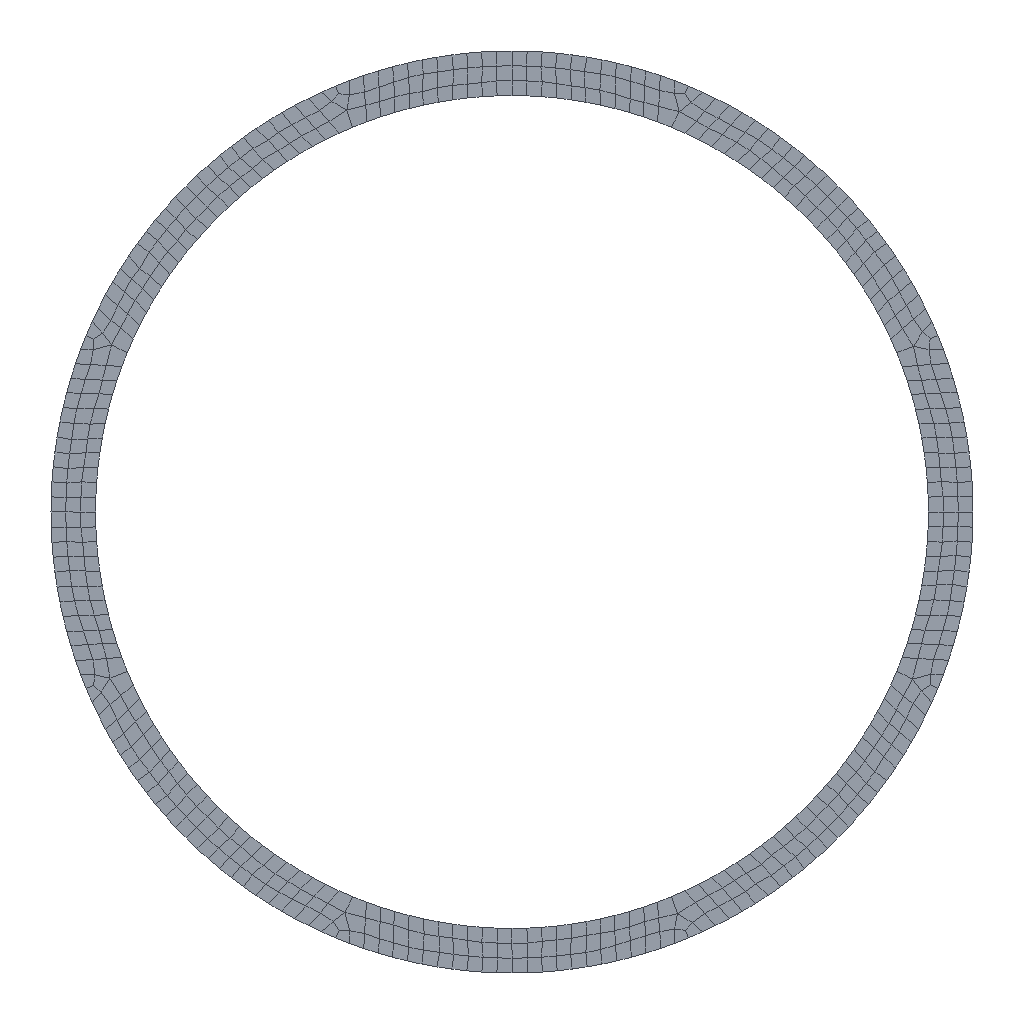Simulation study | ansys workbench
Set-up summary:
category,name,step,type,value,unit,region
solver,ansys_workbench
units,mm-N-s-tonne (MPa),,stated,"/units,MPA"
analysis,LS1,,static
load_step,LS1,LS1,static,nsubst=1; time=1
mesh,nodes,,,2024
mesh,elements,,,936
element_type,PLANE183,,,552
element_type,SURF153,,,384
material,?,,E,34500,tonne s^-2 mm^-1
material,?,,nu,0.2
material,?,,density,2.5e-09,tonne mm^-3
load,Define Pressure Using Surface Effect Elements,LS1,pressure,3,,SURF153 #3
load,Define Pressure Using Surface Effect Elements,LS1,pressure,3,,SURF153 #4
load,Define Pressure Using Surface Effect Elements,LS1,pressure,4,,SURF153 #5
load,Define Pressure Using Surface Effect Elements,LS1,pressure,4,,SURF153 #6
bc,Constant Zero Displacement X,model,fixed,[dofs=UX],,_DISPZEROUX
bc,Constant Zero Displacement Y,model,fixed,[dofs=UY],,_DISPZEROUY
named_set,_DISPZEROUX,,node,1
named_set,_DISPZEROUY,,node,1
Ansys APDL input file, long lists of numbers shortened:
/batch
/config,noeldb,1     ! force off writing results to database
*get,_wallstrt,active,,time,wall
! ANSYS input file written by Workbench version 2021 R1
! File used for geometry attach:
/title,____--____ (B5)
! ****** Begin Custom Load Command Snippet ******
/COM, ACT Extensions:
/COM,     LSDYNA, 2021.1
/COM,
! ****** End   Custom Load Command Snippet ******
*DIM,_wb_ProjectScratch_dir,string,248
_wb_ProjectScratch_dir(1) = ''
*DIM,_wb_SolverFiles_dir,string,248
_wb_SolverFiles_dir(1) = ''
*DIM,_wb_userfiles_dir,string,248
_wb_userfiles_dir(1) = ''
/com,--- Data in consistent NMM units. See Solving Units in the help system for more information.
/units,MPA
/nopr
/wb,file,start              !  signify a WB generated input file
/prep7
! Turn off shape checking because checks already performed inside WB mesher.
! See help system for more information.
SHPP,OFF,,NOWARN
/nolist
etcon,set             ! allow ANSYS to choose best KEYOP's for 180x elements, resets any applicable keyopt to MAPDL defaults
/com,*********** Nodes for the whole assembly ***********
nblock,3,,2226
(1i9,3e20.9e3)
        1     0.000000000E+00     3.100000000E+03     0.000000000E+00
! (2023 more lines like these left out)
-1
/wb,elem,start            !  set before creation of elements
/com,*********** Elements for Body 1 "____3-FreeParts|NONE" ***********
et,1,183
keyo,1,3,3
eblock,19,solid,,552
(19i9)
        1        1        1        1        0        0        0        0        8        0        1      702      701      725      724     1978     1979     2014     1981
! (551 more lines like these left out)
-1
/wb,elem,end               !  done creating elements
/com,*********** Send User Defined Coordinate System(s) ***********
csys,0
toffst,273.15,  ! Temperature offset from absolute zero
/com,*********** Set Reference Temperature ***********
tref,22.
/wb,mat,start              !  starting to send materials
/com,*********** Send Materials ***********
MP,DENS,1,2.5e-09,	! tonne mm^-3
MP,EX,1,34500,	! tonne s^-2 mm^-1
MP,NUXY,1,0.2,
/wb,mat,end                !  done sending materials
/com,*********** Send Sheet Properties ***********
r,1,100.
!************************* Model Summary ********************
!____3-FreeParts|NONE,	支护,	matid,	1
!************************* End Model Summary ********************
! get the diagonal of the bounding box. Needed later for other things
*get,_xmin,node,,mnloc,x
*get,_ymin,node,,mnloc,y
*get,_zmin,node,,mnloc,z
*get,_xmax,node,,mxloc,x
*get,_ymax,node,,mxloc,y
*get,_zmax,node,,mxloc,z
_ASMDIAG=(_xmax-_xmin)*(_xmax-_xmin)+(_ymax-_ymin)*(_ymax-_ymin)+(_zmax-_zmin)*(_zmax-_zmin)
_ASMDIAG=SQRT(_ASMDIAG)
/wb,contact,start          !  starting to send contact
/wb,contact,end            !  done creating contacts
/golist
/wb,load,start             !  starting to send loads
/com,******* Constant Zero Displacement X *******
CMBLOCK,_DISPZEROUX,NODE,        1
(8i10)
       317
cmsel,s,_DISPZEROUX
d,all,ux,0
nsel,all
/com,******* Constant Zero Displacement Y *******
CMBLOCK,_DISPZEROUY,NODE,        1
(8i10)
       317
cmsel,s,_DISPZEROUY
d,all,uy,0
nsel,all
/com,*********** Create Elastic Support ***********
et,2,153
keyop,2,3,10        ! get plane stress option and thickness from underlying element
eblock,10,,,192
(15i9)
      553        2        2        2        0      220      219     1181
! (191 more lines like these left out)
-1
esel,s,type,,2
r,2,,,,5.e-002
esel,all
/com,*********** Define Pressure Using Surface Effect Elements ***********
et,3,153
keyop,3,3,10        ! get plane stress option and thickness from underlying element
eblock,10,,,48
(15i9)
      745        3        3        3        0        2       25      740
! (47 more lines like these left out)
-1
esel,s,type,,3
keyop,3,7,0                ! Use deformed area for application of load
esel,all
/com,*********** Define Pressure Using Surface Effect Elements ***********
et,4,153
keyop,4,3,10        ! get plane stress option and thickness from underlying element
eblock,10,,,48
(15i9)
      793        4        4        4        0      363      362     1469
! (47 more lines like these left out)
-1
esel,s,type,,4
keyop,4,7,0                ! Use deformed area for application of load
esel,all
/com,*********** Define Pressure Using Surface Effect Elements ***********
et,5,153
keyop,5,3,10        ! get plane stress option and thickness from underlying element
eblock,10,,,48
(15i9)
      841        5        5        5        0      220      219     1181
! (47 more lines like these left out)
-1
esel,s,type,,5
keyop,5,7,0                ! Use deformed area for application of load
esel,all
/com,*********** Define Pressure Using Surface Effect Elements ***********
et,6,153
keyop,6,3,10        ! get plane stress option and thickness from underlying element
eblock,10,,,48
(15i9)
      889        6        6        6        0      124      123      987
! (47 more lines like these left out)
-1
esel,s,type,,6
keyop,6,7,0                ! Use deformed area for application of load
esel,all
esel,all
/gst,on,on
fini
*get,_numnode,node,0,count
*get,_numelem,elem,0,count
*get, _MAXELEMNUM, elem, 0, NUM, MAX
*get, _MAXNODENUM, node, 0, NUM, MAX
*get, _MAXELEMTYPE, etyp, 0, NUM, MAX
*get, _MAXREALCONST, real, 0, NUM, MAX
/go
/wb,load,end               !  done creating loads
/com,--- Number of total nodes = %_numnode%
/com,--- Number of contact elements = 384
/com,--- Number of spring elements = 0
/com,--- Number of bearing elements = 0
/com,--- Number of solid elements = 552
/com,--- Number of condensed parts = 0
/com,--- Number of total elements = %_numelem%
*get,_wallbsol,active,,time,wall
/com,****************************************************************************
/com,*************************    SOLUTION       ********************************
/com,****************************************************************************
/solu
antype,0                   ! static analysis
_thickRatio=  0     ! Ratio of thick parts in the model
eqsl,sparse,,,,,1
cntr,print,1               ! print out contact info and also make no initial contact an error
dmpoption,emat,no             ! Don't combine emat file for DANSYS
dmpoption,esav,no             ! Don't combine esav file for DANSYS
nldiag,cont,iter           ! print out contact info each equilibrium iteration
rescontrol,,none                 ! Do not keep any restart files
/com,****************************************************
/com,******************* SOLVE FOR LS 1 OF 1 ****************
esel,s,type,,3
nsle
sf,all,pres,3.
esel,s,type,,4
nsle
sf,all,pres,3.
esel,s,type,,5
nsle
sf,all,pres,4.
esel,s,type,,6
nsle
sf,all,pres,4.
nsel,all
esel,all
acel,0.,9806.65
esel,all
/nopr
/gopr
/nolist
nsub,1,1,1
time,1.
outres,erase
outres,all,none
outres,nsol,all,
outres,rsol,all
outres,eangl,all
outres,etmp,all
outres,veng,all
outres,strs,all,
outres,epel,all,
outres,eppl,all,
outres,cont,all,
! *********** WB SOLVE COMMAND ***********
! check interactive state
*get,ANSINTER_,active,,int
*if,ANSINTER_,ne,0,then
/eof
*endif
solve
/com *************** Write FE CONNECTORS *********
CEWRITE,file,ce,,INTE
/com,****************************************************
/com,*************** FINISHED SOLVE FOR LS 1 *************
*get,_wallasol,active,,time,wall
/nopr
*get,_numnode,node,0,count
*get,_numelem,elem,0,count
*get, _MAXELEMNUM, elem, 0, NUM, MAX
*get, _MAXNODENUM, node, 0, NUM, MAX,,,INTERNAL
*get, _MAXELEMTYPE, etyp, 0, NUM, MAX
*get, _MAXREALCONST, real, 0, NUM, MAX
/gopr
/post1
xmlo,ENCODING,ISO-8859-1
xmlo,parm
/xml,parm,xml
fini
/gopr
*get,_walldone,active,,time,wall
_preptime=(_wallbsol-_wallstrt)*3600
_solvtime=(_wallasol-_wallbsol)*3600
_posttime=(_walldone-_wallasol)*3600
_totaltim=(_walldone-_wallstrt)*3600
*get,_dlbratio,active,0,solu,dlbr
*get,_combtime,active,0,solu,comb
/com,--- Total number of nodes = %_numnode%
/com,--- Total number of elements = %_numelem%
/com,--- Element load balance ratio = %_dlbratio%
/com,--- Time to combine distributed files = %_combtime%
/wb,file,end               ! done with WB generated input
Results summary:
result,analyses[0].index,,,1
result,analyses[0].system,,,SYS-1
result,analyses[0].deck,,,deck.dat
result,analyses[0].solve_status,,,completed
result,analyses[0].analysis_type,,,static
result,analyses[0].physics,,,mechanical
result,analyses[0].unit_system,,,"NMM: mm, ton, N, s, mV, mA, degC"
result,analyses[0].n_sets,,,1
result,analyses[0].load_steps[0].set,set=1,,1
result,analyses[0].load_steps[0].time_or_freq,set=1,,1
result,analyses[0].load_steps[0].max_displacement_magnitude,set=1,,11.947
result,analyses[0].load_steps[0].max_von_mises_nodal,set=1,,57.664
result,analyses[0].load_steps[0].reaction_force_sum_xyz[1],set=1,,2.82168e-06
result,analyses[0].load_steps[0].reaction_force_sum_xyz[2],set=1,,142048
result,analyses[0].load_steps[0].reaction_force_sum_xyz[3],set=1,,0
result,geometry_export[0][0],,,.step
result,geometry_export[0][1],,,ok
result,geometry_export[0][2],,,1